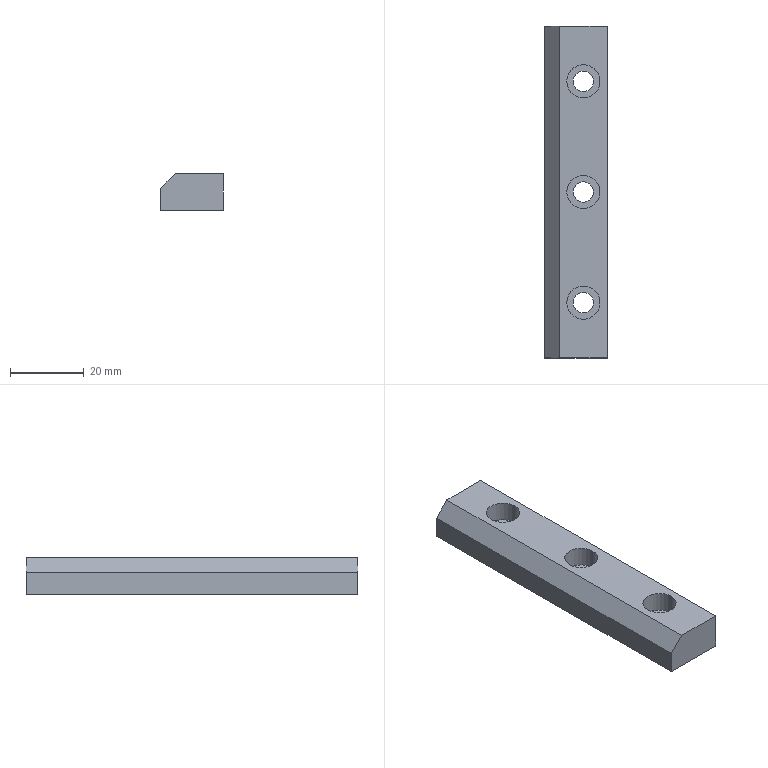Part | STEP file | slide seat cover plate 4 | 1 solid | 22 faces | box 17 x 90 x 10 mm | volume 13210 mm3 | cylinder 12 | plane 10 | commonest cylinder face diameters 5.5 x6 9 x6
STEP:
#1=CARTESIAN_POINT('',(0.,0.,0.));
#2=DIRECTION('',(0.,0.,1.));
#3=DIRECTION('',(1.,0.,0.));
#4=AXIS2_PLACEMENT_3D('',#1,#2,#3);
#5=CARTESIAN_POINT('',(8.148,22.1,4.5));
#6=VERTEX_POINT('',#5);
#7=CARTESIAN_POINT('',(8.148,22.1,10.));
#8=VERTEX_POINT('',#7);
#9=CARTESIAN_POINT('',(8.148,22.1,4.5));
#10=DIRECTION('',(0.,0.,1.));
#11=VECTOR('',#10,1.);
#12=LINE('',#9,#11);
#13=CARTESIAN_POINT('',(3.648,22.1,4.5));
#14=DIRECTION('',(0.,0.,1.));
#15=DIRECTION('',(1.,0.,0.));
#16=AXIS2_PLACEMENT_3D('',#13,#14,#15);
#17=CYLINDRICAL_SURFACE('',#16,4.5);
#18=CARTESIAN_POINT('',(6.283,0.));
#19=DIRECTION('',(0.,1.));
#20=VECTOR('',#19,1.);
#21=LINE('',#18,#20);
#22=(GEOMETRIC_REPRESENTATION_CONTEXT(2)PARAMETRIC_REPRESENTATION_CONTEXT()REPRESENTATION_CONTEXT('',''));
#23=DEFINITIONAL_REPRESENTATION('',(#21),#22);
#24=PCURVE('',#17,#23);
#25=CARTESIAN_POINT('',(3.648,22.1,4.5));
#26=DIRECTION('',(0.,0.,1.));
#27=DIRECTION('',(1.,0.,0.));
#28=AXIS2_PLACEMENT_3D('',#25,#26,#27);
#29=CYLINDRICAL_SURFACE('',#28,4.5);
#30=CARTESIAN_POINT('',(0.,0.));
#31=DIRECTION('',(0.,1.));
#32=VECTOR('',#31,1.);
#33=LINE('',#30,#32);
#34=(GEOMETRIC_REPRESENTATION_CONTEXT(2)PARAMETRIC_REPRESENTATION_CONTEXT()REPRESENTATION_CONTEXT('',''));
#35=DEFINITIONAL_REPRESENTATION('',(#33),#34);
#36=PCURVE('',#29,#35);
#37=SURFACE_CURVE('',#12,(#24,#36),.PCURVE_S1.);
#38=EDGE_CURVE('',#6,#8,#37,.T.);
#39=ORIENTED_EDGE('',*,*,#38,.T.);
#40=CARTESIAN_POINT('',(-0.8518,22.1,10.));
#41=VERTEX_POINT('',#40);
#42=CARTESIAN_POINT('',(3.648,22.1,10.));
#43=DIRECTION('',(0.,0.,1.));
#44=DIRECTION('',(1.,0.,0.));
#45=AXIS2_PLACEMENT_3D('',#42,#43,#44);
#46=CIRCLE('',#45,4.5);
#47=CARTESIAN_POINT('',(0.,5.5));
#48=DIRECTION('',(1.,0.));
#49=VECTOR('',#48,1.);
#50=LINE('',#47,#49);
#51=(GEOMETRIC_REPRESENTATION_CONTEXT(2)PARAMETRIC_REPRESENTATION_CONTEXT()REPRESENTATION_CONTEXT('',''));
#52=DEFINITIONAL_REPRESENTATION('',(#50),#51);
#53=PCURVE('',#17,#52);
#54=CARTESIAN_POINT('',(-6.852,-52.9,10.));
#55=DIRECTION('',(0.,0.,1.));
#56=DIRECTION('',(1.,0.,0.));
#57=AXIS2_PLACEMENT_3D('',#54,#55,#56);
#58=PLANE('',#57);
#59=CARTESIAN_POINT('',(10.5,75.));
#60=DIRECTION('',(1.,0.));
#61=AXIS2_PLACEMENT_2D('',#59,#60);
#62=CIRCLE('',#61,4.5);
#63=(GEOMETRIC_REPRESENTATION_CONTEXT(2)PARAMETRIC_REPRESENTATION_CONTEXT()REPRESENTATION_CONTEXT('',''));
#64=DEFINITIONAL_REPRESENTATION('',(#62),#63);
#65=PCURVE('',#58,#64);
#66=SURFACE_CURVE('',#46,(#53,#65),.PCURVE_S1.);
#67=EDGE_CURVE('',#41,#8,#66,.T.);
#68=ORIENTED_EDGE('',*,*,#67,.F.);
#69=CARTESIAN_POINT('',(-0.8518,22.1,4.5));
#70=VERTEX_POINT('',#69);
#71=CARTESIAN_POINT('',(-0.8518,22.1,4.5));
#72=DIRECTION('',(0.,0.,1.));
#73=VECTOR('',#72,1.);
#74=LINE('',#71,#73);
#75=CARTESIAN_POINT('',(3.142,0.));
#76=DIRECTION('',(0.,1.));
#77=VECTOR('',#76,1.);
#78=LINE('',#75,#77);
#79=(GEOMETRIC_REPRESENTATION_CONTEXT(2)PARAMETRIC_REPRESENTATION_CONTEXT()REPRESENTATION_CONTEXT('',''));
#80=DEFINITIONAL_REPRESENTATION('',(#78),#79);
#81=PCURVE('',#17,#80);
#82=CARTESIAN_POINT('',(3.142,0.));
#83=DIRECTION('',(0.,1.));
#84=VECTOR('',#83,1.);
#85=LINE('',#82,#84);
#86=(GEOMETRIC_REPRESENTATION_CONTEXT(2)PARAMETRIC_REPRESENTATION_CONTEXT()REPRESENTATION_CONTEXT('',''));
#87=DEFINITIONAL_REPRESENTATION('',(#85),#86);
#88=PCURVE('',#29,#87);
#89=SURFACE_CURVE('',#74,(#81,#88),.PCURVE_S1.);
#90=EDGE_CURVE('',#70,#41,#89,.T.);
#91=ORIENTED_EDGE('',*,*,#90,.F.);
#92=CARTESIAN_POINT('',(3.648,22.1,4.5));
#93=DIRECTION('',(0.,0.,1.));
#94=DIRECTION('',(1.,0.,0.));
#95=AXIS2_PLACEMENT_3D('',#92,#93,#94);
#96=CIRCLE('',#95,4.5);
#97=CARTESIAN_POINT('',(0.,0.));
#98=DIRECTION('',(1.,0.));
#99=VECTOR('',#98,1.);
#100=LINE('',#97,#99);
#101=(GEOMETRIC_REPRESENTATION_CONTEXT(2)PARAMETRIC_REPRESENTATION_CONTEXT()REPRESENTATION_CONTEXT('',''));
#102=DEFINITIONAL_REPRESENTATION('',(#100),#101);
#103=PCURVE('',#17,#102);
#104=CARTESIAN_POINT('',(3.648,22.1,4.5));
#105=DIRECTION('',(0.,0.,1.));
#106=DIRECTION('',(1.,0.,0.));
#107=AXIS2_PLACEMENT_3D('',#104,#105,#106);
#108=PLANE('',#107);
#109=CARTESIAN_POINT('',(0.,0.));
#110=DIRECTION('',(1.,0.));
#111=AXIS2_PLACEMENT_2D('',#109,#110);
#112=CIRCLE('',#111,4.5);
#113=(GEOMETRIC_REPRESENTATION_CONTEXT(2)PARAMETRIC_REPRESENTATION_CONTEXT()REPRESENTATION_CONTEXT('',''));
#114=DEFINITIONAL_REPRESENTATION('',(#112),#113);
#115=PCURVE('',#108,#114);
#116=SURFACE_CURVE('',#96,(#103,#115),.PCURVE_S1.);
#117=EDGE_CURVE('',#70,#6,#116,.T.);
#118=ORIENTED_EDGE('',*,*,#117,.T.);
#119=EDGE_LOOP('',(#39,#68,#91,#118));
#120=FACE_BOUND('',#119,.F.);
#121=ADVANCED_FACE('',(#120),#17,.F.);
#122=CARTESIAN_POINT('',(8.148,-7.9,4.5));
#123=VERTEX_POINT('',#122);
#124=CARTESIAN_POINT('',(8.148,-7.9,10.));
#125=VERTEX_POINT('',#124);
#126=CARTESIAN_POINT('',(8.148,-7.9,4.5));
#127=DIRECTION('',(0.,0.,1.));
#128=VECTOR('',#127,1.);
#129=LINE('',#126,#128);
#130=CARTESIAN_POINT('',(3.648,-7.9,4.5));
#131=DIRECTION('',(0.,0.,1.));
#132=DIRECTION('',(1.,0.,0.));
#133=AXIS2_PLACEMENT_3D('',#130,#131,#132);
#134=CYLINDRICAL_SURFACE('',#133,4.5);
#135=CARTESIAN_POINT('',(6.283,0.));
#136=DIRECTION('',(0.,1.));
#137=VECTOR('',#136,1.);
#138=LINE('',#135,#137);
#139=(GEOMETRIC_REPRESENTATION_CONTEXT(2)PARAMETRIC_REPRESENTATION_CONTEXT()REPRESENTATION_CONTEXT('',''));
#140=DEFINITIONAL_REPRESENTATION('',(#138),#139);
#141=PCURVE('',#134,#140);
#142=CARTESIAN_POINT('',(3.648,-7.9,4.5));
#143=DIRECTION('',(0.,0.,1.));
#144=DIRECTION('',(1.,0.,0.));
#145=AXIS2_PLACEMENT_3D('',#142,#143,#144);
#146=CYLINDRICAL_SURFACE('',#145,4.5);
#147=CARTESIAN_POINT('',(0.,0.));
#148=DIRECTION('',(0.,1.));
#149=VECTOR('',#148,1.);
#150=LINE('',#147,#149);
#151=(GEOMETRIC_REPRESENTATION_CONTEXT(2)PARAMETRIC_REPRESENTATION_CONTEXT()REPRESENTATION_CONTEXT('',''));
#152=DEFINITIONAL_REPRESENTATION('',(#150),#151);
#153=PCURVE('',#146,#152);
#154=SURFACE_CURVE('',#129,(#141,#153),.PCURVE_S1.);
#155=EDGE_CURVE('',#123,#125,#154,.T.);
#156=ORIENTED_EDGE('',*,*,#155,.T.);
#157=CARTESIAN_POINT('',(-0.8518,-7.9,10.));
#158=VERTEX_POINT('',#157);
#159=CARTESIAN_POINT('',(3.648,-7.9,10.));
#160=DIRECTION('',(0.,0.,1.));
#161=DIRECTION('',(1.,0.,0.));
#162=AXIS2_PLACEMENT_3D('',#159,#160,#161);
#163=CIRCLE('',#162,4.5);
#164=CARTESIAN_POINT('',(0.,5.5));
#165=DIRECTION('',(1.,0.));
#166=VECTOR('',#165,1.);
#167=LINE('',#164,#166);
#168=(GEOMETRIC_REPRESENTATION_CONTEXT(2)PARAMETRIC_REPRESENTATION_CONTEXT()REPRESENTATION_CONTEXT('',''));
#169=DEFINITIONAL_REPRESENTATION('',(#167),#168);
#170=PCURVE('',#134,#169);
#171=CARTESIAN_POINT('',(10.5,45.));
#172=DIRECTION('',(1.,0.));
#173=AXIS2_PLACEMENT_2D('',#171,#172);
#174=CIRCLE('',#173,4.5);
#175=(GEOMETRIC_REPRESENTATION_CONTEXT(2)PARAMETRIC_REPRESENTATION_CONTEXT()REPRESENTATION_CONTEXT('',''));
#176=DEFINITIONAL_REPRESENTATION('',(#174),#175);
#177=PCURVE('',#58,#176);
#178=SURFACE_CURVE('',#163,(#170,#177),.PCURVE_S1.);
#179=EDGE_CURVE('',#158,#125,#178,.T.);
#180=ORIENTED_EDGE('',*,*,#179,.F.);
#181=CARTESIAN_POINT('',(-0.8518,-7.9,4.5));
#182=VERTEX_POINT('',#181);
#183=CARTESIAN_POINT('',(-0.8518,-7.9,4.5));
#184=DIRECTION('',(0.,0.,1.));
#185=VECTOR('',#184,1.);
#186=LINE('',#183,#185);
#187=CARTESIAN_POINT('',(3.142,0.));
#188=DIRECTION('',(0.,1.));
#189=VECTOR('',#188,1.);
#190=LINE('',#187,#189);
#191=(GEOMETRIC_REPRESENTATION_CONTEXT(2)PARAMETRIC_REPRESENTATION_CONTEXT()REPRESENTATION_CONTEXT('',''));
#192=DEFINITIONAL_REPRESENTATION('',(#190),#191);
#193=PCURVE('',#134,#192);
#194=CARTESIAN_POINT('',(3.142,0.));
#195=DIRECTION('',(0.,1.));
#196=VECTOR('',#195,1.);
#197=LINE('',#194,#196);
#198=(GEOMETRIC_REPRESENTATION_CONTEXT(2)PARAMETRIC_REPRESENTATION_CONTEXT()REPRESENTATION_CONTEXT('',''));
#199=DEFINITIONAL_REPRESENTATION('',(#197),#198);
#200=PCURVE('',#146,#199);
#201=SURFACE_CURVE('',#186,(#193,#200),.PCURVE_S1.);
#202=EDGE_CURVE('',#182,#158,#201,.T.);
#203=ORIENTED_EDGE('',*,*,#202,.F.);
#204=CARTESIAN_POINT('',(3.648,-7.9,4.5));
#205=DIRECTION('',(0.,0.,1.));
#206=DIRECTION('',(1.,0.,0.));
#207=AXIS2_PLACEMENT_3D('',#204,#205,#206);
#208=CIRCLE('',#207,4.5);
#209=CARTESIAN_POINT('',(0.,0.));
#210=DIRECTION('',(1.,0.));
#211=VECTOR('',#210,1.);
#212=LINE('',#209,#211);
#213=(GEOMETRIC_REPRESENTATION_CONTEXT(2)PARAMETRIC_REPRESENTATION_CONTEXT()REPRESENTATION_CONTEXT('',''));
#214=DEFINITIONAL_REPRESENTATION('',(#212),#213);
#215=PCURVE('',#134,#214);
#216=CARTESIAN_POINT('',(3.648,-7.9,4.5));
#217=DIRECTION('',(0.,0.,1.));
#218=DIRECTION('',(1.,0.,0.));
#219=AXIS2_PLACEMENT_3D('',#216,#217,#218);
#220=PLANE('',#219);
#221=CARTESIAN_POINT('',(0.,0.));
#222=DIRECTION('',(1.,0.));
#223=AXIS2_PLACEMENT_2D('',#221,#222);
#224=CIRCLE('',#223,4.5);
#225=(GEOMETRIC_REPRESENTATION_CONTEXT(2)PARAMETRIC_REPRESENTATION_CONTEXT()REPRESENTATION_CONTEXT('',''));
#226=DEFINITIONAL_REPRESENTATION('',(#224),#225);
#227=PCURVE('',#220,#226);
#228=SURFACE_CURVE('',#208,(#215,#227),.PCURVE_S1.);
#229=EDGE_CURVE('',#182,#123,#228,.T.);
#230=ORIENTED_EDGE('',*,*,#229,.T.);
#231=EDGE_LOOP('',(#156,#180,#203,#230));
#232=FACE_BOUND('',#231,.F.);
#233=ADVANCED_FACE('',(#232),#134,.F.);
#234=CARTESIAN_POINT('',(8.148,-37.9,4.5));
#235=VERTEX_POINT('',#234);
#236=CARTESIAN_POINT('',(8.148,-37.9,10.));
#237=VERTEX_POINT('',#236);
#238=CARTESIAN_POINT('',(8.148,-37.9,4.5));
#239=DIRECTION('',(0.,0.,1.));
#240=VECTOR('',#239,1.);
#241=LINE('',#238,#240);
#242=CARTESIAN_POINT('',(3.648,-37.9,4.5));
#243=DIRECTION('',(0.,0.,1.));
#244=DIRECTION('',(1.,0.,0.));
#245=AXIS2_PLACEMENT_3D('',#242,#243,#244);
#246=CYLINDRICAL_SURFACE('',#245,4.5);
#247=CARTESIAN_POINT('',(6.283,0.));
#248=DIRECTION('',(0.,1.));
#249=VECTOR('',#248,1.);
#250=LINE('',#247,#249);
#251=(GEOMETRIC_REPRESENTATION_CONTEXT(2)PARAMETRIC_REPRESENTATION_CONTEXT()REPRESENTATION_CONTEXT('',''));
#252=DEFINITIONAL_REPRESENTATION('',(#250),#251);
#253=PCURVE('',#246,#252);
#254=CARTESIAN_POINT('',(3.648,-37.9,4.5));
#255=DIRECTION('',(0.,0.,1.));
#256=DIRECTION('',(1.,0.,0.));
#257=AXIS2_PLACEMENT_3D('',#254,#255,#256);
#258=CYLINDRICAL_SURFACE('',#257,4.5);
#259=CARTESIAN_POINT('',(0.,0.));
#260=DIRECTION('',(0.,1.));
#261=VECTOR('',#260,1.);
#262=LINE('',#259,#261);
#263=(GEOMETRIC_REPRESENTATION_CONTEXT(2)PARAMETRIC_REPRESENTATION_CONTEXT()REPRESENTATION_CONTEXT('',''));
#264=DEFINITIONAL_REPRESENTATION('',(#262),#263);
#265=PCURVE('',#258,#264);
#266=SURFACE_CURVE('',#241,(#253,#265),.PCURVE_S1.);
#267=EDGE_CURVE('',#235,#237,#266,.T.);
#268=ORIENTED_EDGE('',*,*,#267,.T.);
#269=CARTESIAN_POINT('',(-0.8518,-37.9,10.));
#270=VERTEX_POINT('',#269);
#271=CARTESIAN_POINT('',(3.648,-37.9,10.));
#272=DIRECTION('',(0.,0.,1.));
#273=DIRECTION('',(1.,0.,0.));
#274=AXIS2_PLACEMENT_3D('',#271,#272,#273);
#275=CIRCLE('',#274,4.5);
#276=CARTESIAN_POINT('',(0.,5.5));
#277=DIRECTION('',(1.,0.));
#278=VECTOR('',#277,1.);
#279=LINE('',#276,#278);
#280=(GEOMETRIC_REPRESENTATION_CONTEXT(2)PARAMETRIC_REPRESENTATION_CONTEXT()REPRESENTATION_CONTEXT('',''));
#281=DEFINITIONAL_REPRESENTATION('',(#279),#280);
#282=PCURVE('',#246,#281);
#283=CARTESIAN_POINT('',(10.5,15.));
#284=DIRECTION('',(1.,0.));
#285=AXIS2_PLACEMENT_2D('',#283,#284);
#286=CIRCLE('',#285,4.5);
#287=(GEOMETRIC_REPRESENTATION_CONTEXT(2)PARAMETRIC_REPRESENTATION_CONTEXT()REPRESENTATION_CONTEXT('',''));
#288=DEFINITIONAL_REPRESENTATION('',(#286),#287);
#289=PCURVE('',#58,#288);
#290=SURFACE_CURVE('',#275,(#282,#289),.PCURVE_S1.);
#291=EDGE_CURVE('',#270,#237,#290,.T.);
#292=ORIENTED_EDGE('',*,*,#291,.F.);
#293=CARTESIAN_POINT('',(-0.8518,-37.9,4.5));
#294=VERTEX_POINT('',#293);
#295=CARTESIAN_POINT('',(-0.8518,-37.9,4.5));
#296=DIRECTION('',(0.,0.,1.));
#297=VECTOR('',#296,1.);
#298=LINE('',#295,#297);
#299=CARTESIAN_POINT('',(3.142,0.));
#300=DIRECTION('',(0.,1.));
#301=VECTOR('',#300,1.);
#302=LINE('',#299,#301);
#303=(GEOMETRIC_REPRESENTATION_CONTEXT(2)PARAMETRIC_REPRESENTATION_CONTEXT()REPRESENTATION_CONTEXT('',''));
#304=DEFINITIONAL_REPRESENTATION('',(#302),#303);
#305=PCURVE('',#246,#304);
#306=CARTESIAN_POINT('',(3.142,0.));
#307=DIRECTION('',(0.,1.));
#308=VECTOR('',#307,1.);
#309=LINE('',#306,#308);
#310=(GEOMETRIC_REPRESENTATION_CONTEXT(2)PARAMETRIC_REPRESENTATION_CONTEXT()REPRESENTATION_CONTEXT('',''));
#311=DEFINITIONAL_REPRESENTATION('',(#309),#310);
#312=PCURVE('',#258,#311);
#313=SURFACE_CURVE('',#298,(#305,#312),.PCURVE_S1.);
#314=EDGE_CURVE('',#294,#270,#313,.T.);
#315=ORIENTED_EDGE('',*,*,#314,.F.);
#316=CARTESIAN_POINT('',(3.648,-37.9,4.5));
#317=DIRECTION('',(0.,0.,1.));
#318=DIRECTION('',(1.,0.,0.));
#319=AXIS2_PLACEMENT_3D('',#316,#317,#318);
#320=CIRCLE('',#319,4.5);
#321=CARTESIAN_POINT('',(0.,0.));
#322=DIRECTION('',(1.,0.));
#323=VECTOR('',#322,1.);
#324=LINE('',#321,#323);
#325=(GEOMETRIC_REPRESENTATION_CONTEXT(2)PARAMETRIC_REPRESENTATION_CONTEXT()REPRESENTATION_CONTEXT('',''));
#326=DEFINITIONAL_REPRESENTATION('',(#324),#325);
#327=PCURVE('',#246,#326);
#328=CARTESIAN_POINT('',(3.648,-37.9,4.5));
#329=DIRECTION('',(0.,0.,1.));
#330=DIRECTION('',(1.,0.,0.));
#331=AXIS2_PLACEMENT_3D('',#328,#329,#330);
#332=PLANE('',#331);
#333=CARTESIAN_POINT('',(0.,0.));
#334=DIRECTION('',(1.,0.));
#335=AXIS2_PLACEMENT_2D('',#333,#334);
#336=CIRCLE('',#335,4.5);
#337=(GEOMETRIC_REPRESENTATION_CONTEXT(2)PARAMETRIC_REPRESENTATION_CONTEXT()REPRESENTATION_CONTEXT('',''));
#338=DEFINITIONAL_REPRESENTATION('',(#336),#337);
#339=PCURVE('',#332,#338);
#340=SURFACE_CURVE('',#320,(#327,#339),.PCURVE_S1.);
#341=EDGE_CURVE('',#294,#235,#340,.T.);
#342=ORIENTED_EDGE('',*,*,#341,.T.);
#343=EDGE_LOOP('',(#268,#292,#315,#342));
#344=FACE_BOUND('',#343,.F.);
#345=ADVANCED_FACE('',(#344),#246,.F.);
#346=CARTESIAN_POINT('',(0.8982,-37.9,4.5));
#347=VERTEX_POINT('',#346);
#348=CARTESIAN_POINT('',(0.8982,-37.9,0.));
#349=VERTEX_POINT('',#348);
#350=CARTESIAN_POINT('',(0.8982,-37.9,10.));
#351=DIRECTION('',(0.,0.,-1.));
#352=VECTOR('',#351,1.);
#353=LINE('',#350,#352);
#354=CARTESIAN_POINT('',(3.648,-37.9,10.));
#355=DIRECTION('',(0.,0.,-1.));
#356=DIRECTION('',(-1.,0.,0.));
#357=AXIS2_PLACEMENT_3D('',#354,#355,#356);
#358=CYLINDRICAL_SURFACE('',#357,2.75);
#359=CARTESIAN_POINT('',(6.283,0.));
#360=DIRECTION('',(0.,1.));
#361=VECTOR('',#360,1.);
#362=LINE('',#359,#361);
#363=(GEOMETRIC_REPRESENTATION_CONTEXT(2)PARAMETRIC_REPRESENTATION_CONTEXT()REPRESENTATION_CONTEXT('',''));
#364=DEFINITIONAL_REPRESENTATION('',(#362),#363);
#365=PCURVE('',#358,#364);
#366=CARTESIAN_POINT('',(3.648,-37.9,10.));
#367=DIRECTION('',(0.,0.,-1.));
#368=DIRECTION('',(-1.,0.,0.));
#369=AXIS2_PLACEMENT_3D('',#366,#367,#368);
#370=CYLINDRICAL_SURFACE('',#369,2.75);
#371=CARTESIAN_POINT('',(0.,0.));
#372=DIRECTION('',(0.,1.));
#373=VECTOR('',#372,1.);
#374=LINE('',#371,#373);
#375=(GEOMETRIC_REPRESENTATION_CONTEXT(2)PARAMETRIC_REPRESENTATION_CONTEXT()REPRESENTATION_CONTEXT('',''));
#376=DEFINITIONAL_REPRESENTATION('',(#374),#375);
#377=PCURVE('',#370,#376);
#378=SURFACE_CURVE('',#353,(#365,#377),.PCURVE_S1.);
#379=EDGE_CURVE('',#347,#349,#378,.T.);
#380=ORIENTED_EDGE('',*,*,#379,.T.);
#381=CARTESIAN_POINT('',(6.398,-37.9,0.));
#382=VERTEX_POINT('',#381);
#383=CARTESIAN_POINT('',(3.648,-37.9,0.));
#384=DIRECTION('',(0.,0.,1.));
#385=DIRECTION('',(1.,0.,0.));
#386=AXIS2_PLACEMENT_3D('',#383,#384,#385);
#387=CIRCLE('',#386,2.75);
#388=CARTESIAN_POINT('',(9.425,10.));
#389=DIRECTION('',(-1.,0.));
#390=VECTOR('',#389,1.);
#391=LINE('',#388,#390);
#392=(GEOMETRIC_REPRESENTATION_CONTEXT(2)PARAMETRIC_REPRESENTATION_CONTEXT()REPRESENTATION_CONTEXT('',''));
#393=DEFINITIONAL_REPRESENTATION('',(#391),#392);
#394=PCURVE('',#358,#393);
#395=CARTESIAN_POINT('',(-6.852,-52.9,0.));
#396=DIRECTION('',(0.,0.,1.));
#397=DIRECTION('',(1.,0.,0.));
#398=AXIS2_PLACEMENT_3D('',#395,#396,#397);
#399=PLANE('',#398);
#400=CARTESIAN_POINT('',(10.5,15.));
#401=DIRECTION('',(1.,0.));
#402=AXIS2_PLACEMENT_2D('',#400,#401);
#403=CIRCLE('',#402,2.75);
#404=(GEOMETRIC_REPRESENTATION_CONTEXT(2)PARAMETRIC_REPRESENTATION_CONTEXT()REPRESENTATION_CONTEXT('',''));
#405=DEFINITIONAL_REPRESENTATION('',(#403),#404);
#406=PCURVE('',#399,#405);
#407=SURFACE_CURVE('',#387,(#394,#406),.PCURVE_S1.);
#408=EDGE_CURVE('',#349,#382,#407,.T.);
#409=ORIENTED_EDGE('',*,*,#408,.T.);
#410=CARTESIAN_POINT('',(6.398,-37.9,4.5));
#411=VERTEX_POINT('',#410);
#412=CARTESIAN_POINT('',(6.398,-37.9,10.));
#413=DIRECTION('',(0.,0.,-1.));
#414=VECTOR('',#413,1.);
#415=LINE('',#412,#414);
#416=CARTESIAN_POINT('',(3.142,0.));
#417=DIRECTION('',(0.,1.));
#418=VECTOR('',#417,1.);
#419=LINE('',#416,#418);
#420=(GEOMETRIC_REPRESENTATION_CONTEXT(2)PARAMETRIC_REPRESENTATION_CONTEXT()REPRESENTATION_CONTEXT('',''));
#421=DEFINITIONAL_REPRESENTATION('',(#419),#420);
#422=PCURVE('',#358,#421);
#423=CARTESIAN_POINT('',(3.142,0.));
#424=DIRECTION('',(0.,1.));
#425=VECTOR('',#424,1.);
#426=LINE('',#423,#425);
#427=(GEOMETRIC_REPRESENTATION_CONTEXT(2)PARAMETRIC_REPRESENTATION_CONTEXT()REPRESENTATION_CONTEXT('',''));
#428=DEFINITIONAL_REPRESENTATION('',(#426),#427);
#429=PCURVE('',#370,#428);
#430=SURFACE_CURVE('',#415,(#422,#429),.PCURVE_S1.);
#431=EDGE_CURVE('',#411,#382,#430,.T.);
#432=ORIENTED_EDGE('',*,*,#431,.F.);
#433=CARTESIAN_POINT('',(3.648,-37.9,4.5));
#434=DIRECTION('',(0.,0.,1.));
#435=DIRECTION('',(1.,0.,0.));
#436=AXIS2_PLACEMENT_3D('',#433,#434,#435);
#437=CIRCLE('',#436,2.75);
#438=CARTESIAN_POINT('',(9.425,5.5));
#439=DIRECTION('',(-1.,0.));
#440=VECTOR('',#439,1.);
#441=LINE('',#438,#440);
#442=(GEOMETRIC_REPRESENTATION_CONTEXT(2)PARAMETRIC_REPRESENTATION_CONTEXT()REPRESENTATION_CONTEXT('',''));
#443=DEFINITIONAL_REPRESENTATION('',(#441),#442);
#444=PCURVE('',#358,#443);
#445=CARTESIAN_POINT('',(0.,0.));
#446=DIRECTION('',(1.,0.));
#447=AXIS2_PLACEMENT_2D('',#445,#446);
#448=CIRCLE('',#447,2.75);
#449=(GEOMETRIC_REPRESENTATION_CONTEXT(2)PARAMETRIC_REPRESENTATION_CONTEXT()REPRESENTATION_CONTEXT('',''));
#450=DEFINITIONAL_REPRESENTATION('',(#448),#449);
#451=PCURVE('',#332,#450);
#452=SURFACE_CURVE('',#437,(#444,#451),.PCURVE_S1.);
#453=EDGE_CURVE('',#347,#411,#452,.T.);
#454=ORIENTED_EDGE('',*,*,#453,.F.);
#455=EDGE_LOOP('',(#380,#409,#432,#454));
#456=FACE_BOUND('',#455,.F.);
#457=ADVANCED_FACE('',(#456),#358,.F.);
#458=CARTESIAN_POINT('',(0.8982,-7.9,4.5));
#459=VERTEX_POINT('',#458);
#460=CARTESIAN_POINT('',(0.8982,-7.9,0.));
#461=VERTEX_POINT('',#460);
#462=CARTESIAN_POINT('',(0.8982,-7.9,10.));
#463=DIRECTION('',(0.,0.,-1.));
#464=VECTOR('',#463,1.);
#465=LINE('',#462,#464);
#466=CARTESIAN_POINT('',(3.648,-7.9,10.));
#467=DIRECTION('',(0.,0.,-1.));
#468=DIRECTION('',(-1.,0.,0.));
#469=AXIS2_PLACEMENT_3D('',#466,#467,#468);
#470=CYLINDRICAL_SURFACE('',#469,2.75);
#471=CARTESIAN_POINT('',(6.283,0.));
#472=DIRECTION('',(0.,1.));
#473=VECTOR('',#472,1.);
#474=LINE('',#471,#473);
#475=(GEOMETRIC_REPRESENTATION_CONTEXT(2)PARAMETRIC_REPRESENTATION_CONTEXT()REPRESENTATION_CONTEXT('',''));
#476=DEFINITIONAL_REPRESENTATION('',(#474),#475);
#477=PCURVE('',#470,#476);
#478=CARTESIAN_POINT('',(3.648,-7.9,10.));
#479=DIRECTION('',(0.,0.,-1.));
#480=DIRECTION('',(-1.,0.,0.));
#481=AXIS2_PLACEMENT_3D('',#478,#479,#480);
#482=CYLINDRICAL_SURFACE('',#481,2.75);
#483=CARTESIAN_POINT('',(0.,0.));
#484=DIRECTION('',(0.,1.));
#485=VECTOR('',#484,1.);
#486=LINE('',#483,#485);
#487=(GEOMETRIC_REPRESENTATION_CONTEXT(2)PARAMETRIC_REPRESENTATION_CONTEXT()REPRESENTATION_CONTEXT('',''));
#488=DEFINITIONAL_REPRESENTATION('',(#486),#487);
#489=PCURVE('',#482,#488);
#490=SURFACE_CURVE('',#465,(#477,#489),.PCURVE_S1.);
#491=EDGE_CURVE('',#459,#461,#490,.T.);
#492=ORIENTED_EDGE('',*,*,#491,.T.);
#493=CARTESIAN_POINT('',(6.398,-7.9,0.));
#494=VERTEX_POINT('',#493);
#495=CARTESIAN_POINT('',(3.648,-7.9,0.));
#496=DIRECTION('',(0.,0.,1.));
#497=DIRECTION('',(1.,0.,0.));
#498=AXIS2_PLACEMENT_3D('',#495,#496,#497);
#499=CIRCLE('',#498,2.75);
#500=CARTESIAN_POINT('',(9.425,10.));
#501=DIRECTION('',(-1.,0.));
#502=VECTOR('',#501,1.);
#503=LINE('',#500,#502);
#504=(GEOMETRIC_REPRESENTATION_CONTEXT(2)PARAMETRIC_REPRESENTATION_CONTEXT()REPRESENTATION_CONTEXT('',''));
#505=DEFINITIONAL_REPRESENTATION('',(#503),#504);
#506=PCURVE('',#470,#505);
#507=CARTESIAN_POINT('',(10.5,45.));
#508=DIRECTION('',(1.,0.));
#509=AXIS2_PLACEMENT_2D('',#507,#508);
#510=CIRCLE('',#509,2.75);
#511=(GEOMETRIC_REPRESENTATION_CONTEXT(2)PARAMETRIC_REPRESENTATION_CONTEXT()REPRESENTATION_CONTEXT('',''));
#512=DEFINITIONAL_REPRESENTATION('',(#510),#511);
#513=PCURVE('',#399,#512);
#514=SURFACE_CURVE('',#499,(#506,#513),.PCURVE_S1.);
#515=EDGE_CURVE('',#461,#494,#514,.T.);
#516=ORIENTED_EDGE('',*,*,#515,.T.);
#517=CARTESIAN_POINT('',(6.398,-7.9,4.5));
#518=VERTEX_POINT('',#517);
#519=CARTESIAN_POINT('',(6.398,-7.9,10.));
#520=DIRECTION('',(0.,0.,-1.));
#521=VECTOR('',#520,1.);
#522=LINE('',#519,#521);
#523=CARTESIAN_POINT('',(3.142,0.));
#524=DIRECTION('',(0.,1.));
#525=VECTOR('',#524,1.);
#526=LINE('',#523,#525);
#527=(GEOMETRIC_REPRESENTATION_CONTEXT(2)PARAMETRIC_REPRESENTATION_CONTEXT()REPRESENTATION_CONTEXT('',''));
#528=DEFINITIONAL_REPRESENTATION('',(#526),#527);
#529=PCURVE('',#470,#528);
#530=CARTESIAN_POINT('',(3.142,0.));
#531=DIRECTION('',(0.,1.));
#532=VECTOR('',#531,1.);
#533=LINE('',#530,#532);
#534=(GEOMETRIC_REPRESENTATION_CONTEXT(2)PARAMETRIC_REPRESENTATION_CONTEXT()REPRESENTATION_CONTEXT('',''));
#535=DEFINITIONAL_REPRESENTATION('',(#533),#534);
#536=PCURVE('',#482,#535);
#537=SURFACE_CURVE('',#522,(#529,#536),.PCURVE_S1.);
#538=EDGE_CURVE('',#518,#494,#537,.T.);
#539=ORIENTED_EDGE('',*,*,#538,.F.);
#540=CARTESIAN_POINT('',(3.648,-7.9,4.5));
#541=DIRECTION('',(0.,0.,1.));
#542=DIRECTION('',(1.,0.,0.));
#543=AXIS2_PLACEMENT_3D('',#540,#541,#542);
#544=CIRCLE('',#543,2.75);
#545=CARTESIAN_POINT('',(9.425,5.5));
#546=DIRECTION('',(-1.,0.));
#547=VECTOR('',#546,1.);
#548=LINE('',#545,#547);
#549=(GEOMETRIC_REPRESENTATION_CONTEXT(2)PARAMETRIC_REPRESENTATION_CONTEXT()REPRESENTATION_CONTEXT('',''));
#550=DEFINITIONAL_REPRESENTATION('',(#548),#549);
#551=PCURVE('',#470,#550);
#552=CARTESIAN_POINT('',(0.,0.));
#553=DIRECTION('',(1.,0.));
#554=AXIS2_PLACEMENT_2D('',#552,#553);
#555=CIRCLE('',#554,2.75);
#556=(GEOMETRIC_REPRESENTATION_CONTEXT(2)PARAMETRIC_REPRESENTATION_CONTEXT()REPRESENTATION_CONTEXT('',''));
#557=DEFINITIONAL_REPRESENTATION('',(#555),#556);
#558=PCURVE('',#220,#557);
#559=SURFACE_CURVE('',#544,(#551,#558),.PCURVE_S1.);
#560=EDGE_CURVE('',#459,#518,#559,.T.);
#561=ORIENTED_EDGE('',*,*,#560,.F.);
#562=EDGE_LOOP('',(#492,#516,#539,#561));
#563=FACE_BOUND('',#562,.F.);
#564=ADVANCED_FACE('',(#563),#470,.F.);
#565=CARTESIAN_POINT('',(0.8982,22.1,4.5));
#566=VERTEX_POINT('',#565);
#567=CARTESIAN_POINT('',(0.8982,22.1,0.));
#568=VERTEX_POINT('',#567);
#569=CARTESIAN_POINT('',(0.8982,22.1,10.));
#570=DIRECTION('',(0.,0.,-1.));
#571=VECTOR('',#570,1.);
#572=LINE('',#569,#571);
#573=CARTESIAN_POINT('',(3.648,22.1,10.));
#574=DIRECTION('',(0.,0.,-1.));
#575=DIRECTION('',(-1.,0.,0.));
#576=AXIS2_PLACEMENT_3D('',#573,#574,#575);
#577=CYLINDRICAL_SURFACE('',#576,2.75);
#578=CARTESIAN_POINT('',(6.283,0.));
#579=DIRECTION('',(0.,1.));
#580=VECTOR('',#579,1.);
#581=LINE('',#578,#580);
#582=(GEOMETRIC_REPRESENTATION_CONTEXT(2)PARAMETRIC_REPRESENTATION_CONTEXT()REPRESENTATION_CONTEXT('',''));
#583=DEFINITIONAL_REPRESENTATION('',(#581),#582);
#584=PCURVE('',#577,#583);
#585=CARTESIAN_POINT('',(3.648,22.1,10.));
#586=DIRECTION('',(0.,0.,-1.));
#587=DIRECTION('',(-1.,0.,0.));
#588=AXIS2_PLACEMENT_3D('',#585,#586,#587);
#589=CYLINDRICAL_SURFACE('',#588,2.75);
#590=CARTESIAN_POINT('',(0.,0.));
#591=DIRECTION('',(0.,1.));
#592=VECTOR('',#591,1.);
#593=LINE('',#590,#592);
#594=(GEOMETRIC_REPRESENTATION_CONTEXT(2)PARAMETRIC_REPRESENTATION_CONTEXT()REPRESENTATION_CONTEXT('',''));
#595=DEFINITIONAL_REPRESENTATION('',(#593),#594);
#596=PCURVE('',#589,#595);
#597=SURFACE_CURVE('',#572,(#584,#596),.PCURVE_S1.);
#598=EDGE_CURVE('',#566,#568,#597,.T.);
#599=ORIENTED_EDGE('',*,*,#598,.T.);
#600=CARTESIAN_POINT('',(6.398,22.1,0.));
#601=VERTEX_POINT('',#600);
#602=CARTESIAN_POINT('',(3.648,22.1,0.));
#603=DIRECTION('',(0.,0.,1.));
#604=DIRECTION('',(1.,0.,0.));
#605=AXIS2_PLACEMENT_3D('',#602,#603,#604);
#606=CIRCLE('',#605,2.75);
#607=CARTESIAN_POINT('',(9.425,10.));
#608=DIRECTION('',(-1.,0.));
#609=VECTOR('',#608,1.);
#610=LINE('',#607,#609);
#611=(GEOMETRIC_REPRESENTATION_CONTEXT(2)PARAMETRIC_REPRESENTATION_CONTEXT()REPRESENTATION_CONTEXT('',''));
#612=DEFINITIONAL_REPRESENTATION('',(#610),#611);
#613=PCURVE('',#577,#612);
#614=CARTESIAN_POINT('',(10.5,75.));
#615=DIRECTION('',(1.,0.));
#616=AXIS2_PLACEMENT_2D('',#614,#615);
#617=CIRCLE('',#616,2.75);
#618=(GEOMETRIC_REPRESENTATION_CONTEXT(2)PARAMETRIC_REPRESENTATION_CONTEXT()REPRESENTATION_CONTEXT('',''));
#619=DEFINITIONAL_REPRESENTATION('',(#617),#618);
#620=PCURVE('',#399,#619);
#621=SURFACE_CURVE('',#606,(#613,#620),.PCURVE_S1.);
#622=EDGE_CURVE('',#568,#601,#621,.T.);
#623=ORIENTED_EDGE('',*,*,#622,.T.);
#624=CARTESIAN_POINT('',(6.398,22.1,4.5));
#625=VERTEX_POINT('',#624);
#626=CARTESIAN_POINT('',(6.398,22.1,10.));
#627=DIRECTION('',(0.,0.,-1.));
#628=VECTOR('',#627,1.);
#629=LINE('',#626,#628);
#630=CARTESIAN_POINT('',(3.142,0.));
#631=DIRECTION('',(0.,1.));
#632=VECTOR('',#631,1.);
#633=LINE('',#630,#632);
#634=(GEOMETRIC_REPRESENTATION_CONTEXT(2)PARAMETRIC_REPRESENTATION_CONTEXT()REPRESENTATION_CONTEXT('',''));
#635=DEFINITIONAL_REPRESENTATION('',(#633),#634);
#636=PCURVE('',#577,#635);
#637=CARTESIAN_POINT('',(3.142,0.));
#638=DIRECTION('',(0.,1.));
#639=VECTOR('',#638,1.);
#640=LINE('',#637,#639);
#641=(GEOMETRIC_REPRESENTATION_CONTEXT(2)PARAMETRIC_REPRESENTATION_CONTEXT()REPRESENTATION_CONTEXT('',''));
#642=DEFINITIONAL_REPRESENTATION('',(#640),#641);
#643=PCURVE('',#589,#642);
#644=SURFACE_CURVE('',#629,(#636,#643),.PCURVE_S1.);
#645=EDGE_CURVE('',#625,#601,#644,.T.);
#646=ORIENTED_EDGE('',*,*,#645,.F.);
#647=CARTESIAN_POINT('',(3.648,22.1,4.5));
#648=DIRECTION('',(0.,0.,1.));
#649=DIRECTION('',(1.,0.,0.));
#650=AXIS2_PLACEMENT_3D('',#647,#648,#649);
#651=CIRCLE('',#650,2.75);
#652=CARTESIAN_POINT('',(9.425,5.5));
#653=DIRECTION('',(-1.,0.));
#654=VECTOR('',#653,1.);
#655=LINE('',#652,#654);
#656=(GEOMETRIC_REPRESENTATION_CONTEXT(2)PARAMETRIC_REPRESENTATION_CONTEXT()REPRESENTATION_CONTEXT('',''));
#657=DEFINITIONAL_REPRESENTATION('',(#655),#656);
#658=PCURVE('',#577,#657);
#659=CARTESIAN_POINT('',(0.,0.));
#660=DIRECTION('',(1.,0.));
#661=AXIS2_PLACEMENT_2D('',#659,#660);
#662=CIRCLE('',#661,2.75);
#663=(GEOMETRIC_REPRESENTATION_CONTEXT(2)PARAMETRIC_REPRESENTATION_CONTEXT()REPRESENTATION_CONTEXT('',''));
#664=DEFINITIONAL_REPRESENTATION('',(#662),#663);
#665=PCURVE('',#108,#664);
#666=SURFACE_CURVE('',#651,(#658,#665),.PCURVE_S1.);
#667=EDGE_CURVE('',#566,#625,#666,.T.);
#668=ORIENTED_EDGE('',*,*,#667,.F.);
#669=EDGE_LOOP('',(#599,#623,#646,#668));
#670=FACE_BOUND('',#669,.F.);
#671=ADVANCED_FACE('',(#670),#577,.F.);
#672=CARTESIAN_POINT('',(3.648,22.1,0.));
#673=DIRECTION('',(0.,0.,1.));
#674=DIRECTION('',(1.,0.,0.));
#675=AXIS2_PLACEMENT_3D('',#672,#673,#674);
#676=CIRCLE('',#675,2.75);
#677=CARTESIAN_POINT('',(3.142,10.));
#678=DIRECTION('',(-1.,0.));
#679=VECTOR('',#678,1.);
#680=LINE('',#677,#679);
#681=(GEOMETRIC_REPRESENTATION_CONTEXT(2)PARAMETRIC_REPRESENTATION_CONTEXT()REPRESENTATION_CONTEXT('',''));
#682=DEFINITIONAL_REPRESENTATION('',(#680),#681);
#683=PCURVE('',#589,#682);
#684=CARTESIAN_POINT('',(10.5,75.));
#685=DIRECTION('',(1.,0.));
#686=AXIS2_PLACEMENT_2D('',#684,#685);
#687=CIRCLE('',#686,2.75);
#688=(GEOMETRIC_REPRESENTATION_CONTEXT(2)PARAMETRIC_REPRESENTATION_CONTEXT()REPRESENTATION_CONTEXT('',''));
#689=DEFINITIONAL_REPRESENTATION('',(#687),#688);
#690=PCURVE('',#399,#689);
#691=SURFACE_CURVE('',#676,(#683,#690),.PCURVE_S1.);
#692=EDGE_CURVE('',#601,#568,#691,.T.);
#693=ORIENTED_EDGE('',*,*,#692,.T.);
#694=ORIENTED_EDGE('',*,*,#598,.F.);
#695=CARTESIAN_POINT('',(3.648,22.1,4.5));
#696=DIRECTION('',(0.,0.,1.));
#697=DIRECTION('',(1.,0.,0.));
#698=AXIS2_PLACEMENT_3D('',#695,#696,#697);
#699=CIRCLE('',#698,2.75);
#700=CARTESIAN_POINT('',(3.142,5.5));
#701=DIRECTION('',(-1.,0.));
#702=VECTOR('',#701,1.);
#703=LINE('',#700,#702);
#704=(GEOMETRIC_REPRESENTATION_CONTEXT(2)PARAMETRIC_REPRESENTATION_CONTEXT()REPRESENTATION_CONTEXT('',''));
#705=DEFINITIONAL_REPRESENTATION('',(#703),#704);
#706=PCURVE('',#589,#705);
#707=CARTESIAN_POINT('',(0.,0.));
#708=DIRECTION('',(1.,0.));
#709=AXIS2_PLACEMENT_2D('',#707,#708);
#710=CIRCLE('',#709,2.75);
#711=(GEOMETRIC_REPRESENTATION_CONTEXT(2)PARAMETRIC_REPRESENTATION_CONTEXT()REPRESENTATION_CONTEXT('',''));
#712=DEFINITIONAL_REPRESENTATION('',(#710),#711);
#713=PCURVE('',#108,#712);
#714=SURFACE_CURVE('',#699,(#706,#713),.PCURVE_S1.);
#715=EDGE_CURVE('',#625,#566,#714,.T.);
#716=ORIENTED_EDGE('',*,*,#715,.F.);
#717=ORIENTED_EDGE('',*,*,#645,.T.);
#718=EDGE_LOOP('',(#693,#694,#716,#717));
#719=FACE_BOUND('',#718,.F.);
#720=ADVANCED_FACE('',(#719),#589,.F.);
#721=CARTESIAN_POINT('',(3.648,-7.9,0.));
#722=DIRECTION('',(0.,0.,1.));
#723=DIRECTION('',(1.,0.,0.));
#724=AXIS2_PLACEMENT_3D('',#721,#722,#723);
#725=CIRCLE('',#724,2.75);
#726=CARTESIAN_POINT('',(3.142,10.));
#727=DIRECTION('',(-1.,0.));
#728=VECTOR('',#727,1.);
#729=LINE('',#726,#728);
#730=(GEOMETRIC_REPRESENTATION_CONTEXT(2)PARAMETRIC_REPRESENTATION_CONTEXT()REPRESENTATION_CONTEXT('',''));
#731=DEFINITIONAL_REPRESENTATION('',(#729),#730);
#732=PCURVE('',#482,#731);
#733=CARTESIAN_POINT('',(10.5,45.));
#734=DIRECTION('',(1.,0.));
#735=AXIS2_PLACEMENT_2D('',#733,#734);
#736=CIRCLE('',#735,2.75);
#737=(GEOMETRIC_REPRESENTATION_CONTEXT(2)PARAMETRIC_REPRESENTATION_CONTEXT()REPRESENTATION_CONTEXT('',''));
#738=DEFINITIONAL_REPRESENTATION('',(#736),#737);
#739=PCURVE('',#399,#738);
#740=SURFACE_CURVE('',#725,(#732,#739),.PCURVE_S1.);
#741=EDGE_CURVE('',#494,#461,#740,.T.);
#742=ORIENTED_EDGE('',*,*,#741,.T.);
#743=ORIENTED_EDGE('',*,*,#491,.F.);
#744=CARTESIAN_POINT('',(3.648,-7.9,4.5));
#745=DIRECTION('',(0.,0.,1.));
#746=DIRECTION('',(1.,0.,0.));
#747=AXIS2_PLACEMENT_3D('',#744,#745,#746);
#748=CIRCLE('',#747,2.75);
#749=CARTESIAN_POINT('',(3.142,5.5));
#750=DIRECTION('',(-1.,0.));
#751=VECTOR('',#750,1.);
#752=LINE('',#749,#751);
#753=(GEOMETRIC_REPRESENTATION_CONTEXT(2)PARAMETRIC_REPRESENTATION_CONTEXT()REPRESENTATION_CONTEXT('',''));
#754=DEFINITIONAL_REPRESENTATION('',(#752),#753);
#755=PCURVE('',#482,#754);
#756=CARTESIAN_POINT('',(0.,0.));
#757=DIRECTION('',(1.,0.));
#758=AXIS2_PLACEMENT_2D('',#756,#757);
#759=CIRCLE('',#758,2.75);
#760=(GEOMETRIC_REPRESENTATION_CONTEXT(2)PARAMETRIC_REPRESENTATION_CONTEXT()REPRESENTATION_CONTEXT('',''));
#761=DEFINITIONAL_REPRESENTATION('',(#759),#760);
#762=PCURVE('',#220,#761);
#763=SURFACE_CURVE('',#748,(#755,#762),.PCURVE_S1.);
#764=EDGE_CURVE('',#518,#459,#763,.T.);
#765=ORIENTED_EDGE('',*,*,#764,.F.);
#766=ORIENTED_EDGE('',*,*,#538,.T.);
#767=EDGE_LOOP('',(#742,#743,#765,#766));
#768=FACE_BOUND('',#767,.F.);
#769=ADVANCED_FACE('',(#768),#482,.F.);
#770=CARTESIAN_POINT('',(3.648,-37.9,0.));
#771=DIRECTION('',(0.,0.,1.));
#772=DIRECTION('',(1.,0.,0.));
#773=AXIS2_PLACEMENT_3D('',#770,#771,#772);
#774=CIRCLE('',#773,2.75);
#775=CARTESIAN_POINT('',(3.142,10.));
#776=DIRECTION('',(-1.,0.));
#777=VECTOR('',#776,1.);
#778=LINE('',#775,#777);
#779=(GEOMETRIC_REPRESENTATION_CONTEXT(2)PARAMETRIC_REPRESENTATION_CONTEXT()REPRESENTATION_CONTEXT('',''));
#780=DEFINITIONAL_REPRESENTATION('',(#778),#779);
#781=PCURVE('',#370,#780);
#782=CARTESIAN_POINT('',(10.5,15.));
#783=DIRECTION('',(1.,0.));
#784=AXIS2_PLACEMENT_2D('',#782,#783);
#785=CIRCLE('',#784,2.75);
#786=(GEOMETRIC_REPRESENTATION_CONTEXT(2)PARAMETRIC_REPRESENTATION_CONTEXT()REPRESENTATION_CONTEXT('',''));
#787=DEFINITIONAL_REPRESENTATION('',(#785),#786);
#788=PCURVE('',#399,#787);
#789=SURFACE_CURVE('',#774,(#781,#788),.PCURVE_S1.);
#790=EDGE_CURVE('',#382,#349,#789,.T.);
#791=ORIENTED_EDGE('',*,*,#790,.T.);
#792=ORIENTED_EDGE('',*,*,#379,.F.);
#793=CARTESIAN_POINT('',(3.648,-37.9,4.5));
#794=DIRECTION('',(0.,0.,1.));
#795=DIRECTION('',(1.,0.,0.));
#796=AXIS2_PLACEMENT_3D('',#793,#794,#795);
#797=CIRCLE('',#796,2.75);
#798=CARTESIAN_POINT('',(3.142,5.5));
#799=DIRECTION('',(-1.,0.));
#800=VECTOR('',#799,1.);
#801=LINE('',#798,#800);
#802=(GEOMETRIC_REPRESENTATION_CONTEXT(2)PARAMETRIC_REPRESENTATION_CONTEXT()REPRESENTATION_CONTEXT('',''));
#803=DEFINITIONAL_REPRESENTATION('',(#801),#802);
#804=PCURVE('',#370,#803);
#805=CARTESIAN_POINT('',(0.,0.));
#806=DIRECTION('',(1.,0.));
#807=AXIS2_PLACEMENT_2D('',#805,#806);
#808=CIRCLE('',#807,2.75);
#809=(GEOMETRIC_REPRESENTATION_CONTEXT(2)PARAMETRIC_REPRESENTATION_CONTEXT()REPRESENTATION_CONTEXT('',''));
#810=DEFINITIONAL_REPRESENTATION('',(#808),#809);
#811=PCURVE('',#332,#810);
#812=SURFACE_CURVE('',#797,(#804,#811),.PCURVE_S1.);
#813=EDGE_CURVE('',#411,#347,#812,.T.);
#814=ORIENTED_EDGE('',*,*,#813,.F.);
#815=ORIENTED_EDGE('',*,*,#431,.T.);
#816=EDGE_LOOP('',(#791,#792,#814,#815));
#817=FACE_BOUND('',#816,.F.);
#818=ADVANCED_FACE('',(#817),#370,.F.);
#819=CARTESIAN_POINT('',(3.648,22.1,10.));
#820=DIRECTION('',(0.,0.,1.));
#821=DIRECTION('',(1.,0.,0.));
#822=AXIS2_PLACEMENT_3D('',#819,#820,#821);
#823=CIRCLE('',#822,4.5);
#824=CARTESIAN_POINT('',(10.5,75.));
#825=DIRECTION('',(1.,0.));
#826=AXIS2_PLACEMENT_2D('',#824,#825);
#827=CIRCLE('',#826,4.5);
#828=(GEOMETRIC_REPRESENTATION_CONTEXT(2)PARAMETRIC_REPRESENTATION_CONTEXT()REPRESENTATION_CONTEXT('',''));
#829=DEFINITIONAL_REPRESENTATION('',(#827),#828);
#830=PCURVE('',#58,#829);
#831=CARTESIAN_POINT('',(0.,5.5));
#832=DIRECTION('',(1.,0.));
#833=VECTOR('',#832,1.);
#834=LINE('',#831,#833);
#835=(GEOMETRIC_REPRESENTATION_CONTEXT(2)PARAMETRIC_REPRESENTATION_CONTEXT()REPRESENTATION_CONTEXT('',''));
#836=DEFINITIONAL_REPRESENTATION('',(#834),#835);
#837=PCURVE('',#29,#836);
#838=SURFACE_CURVE('',#823,(#830,#837),.PCURVE_S1.);
#839=EDGE_CURVE('',#8,#41,#838,.T.);
#840=ORIENTED_EDGE('',*,*,#839,.F.);
#841=ORIENTED_EDGE('',*,*,#67,.F.);
#842=EDGE_LOOP('',(#840,#841));
#843=FACE_BOUND('',#842,.T.);
#844=CARTESIAN_POINT('',(3.648,-7.9,10.));
#845=DIRECTION('',(0.,0.,1.));
#846=DIRECTION('',(1.,0.,0.));
#847=AXIS2_PLACEMENT_3D('',#844,#845,#846);
#848=CIRCLE('',#847,4.5);
#849=CARTESIAN_POINT('',(10.5,45.));
#850=DIRECTION('',(1.,0.));
#851=AXIS2_PLACEMENT_2D('',#849,#850);
#852=CIRCLE('',#851,4.5);
#853=(GEOMETRIC_REPRESENTATION_CONTEXT(2)PARAMETRIC_REPRESENTATION_CONTEXT()REPRESENTATION_CONTEXT('',''));
#854=DEFINITIONAL_REPRESENTATION('',(#852),#853);
#855=PCURVE('',#58,#854);
#856=CARTESIAN_POINT('',(0.,5.5));
#857=DIRECTION('',(1.,0.));
#858=VECTOR('',#857,1.);
#859=LINE('',#856,#858);
#860=(GEOMETRIC_REPRESENTATION_CONTEXT(2)PARAMETRIC_REPRESENTATION_CONTEXT()REPRESENTATION_CONTEXT('',''));
#861=DEFINITIONAL_REPRESENTATION('',(#859),#860);
#862=PCURVE('',#146,#861);
#863=SURFACE_CURVE('',#848,(#855,#862),.PCURVE_S1.);
#864=EDGE_CURVE('',#125,#158,#863,.T.);
#865=ORIENTED_EDGE('',*,*,#864,.F.);
#866=ORIENTED_EDGE('',*,*,#179,.F.);
#867=EDGE_LOOP('',(#865,#866));
#868=FACE_BOUND('',#867,.T.);
#869=CARTESIAN_POINT('',(3.648,-37.9,10.));
#870=DIRECTION('',(0.,0.,1.));
#871=DIRECTION('',(1.,0.,0.));
#872=AXIS2_PLACEMENT_3D('',#869,#870,#871);
#873=CIRCLE('',#872,4.5);
#874=CARTESIAN_POINT('',(10.5,15.));
#875=DIRECTION('',(1.,0.));
#876=AXIS2_PLACEMENT_2D('',#874,#875);
#877=CIRCLE('',#876,4.5);
#878=(GEOMETRIC_REPRESENTATION_CONTEXT(2)PARAMETRIC_REPRESENTATION_CONTEXT()REPRESENTATION_CONTEXT('',''));
#879=DEFINITIONAL_REPRESENTATION('',(#877),#878);
#880=PCURVE('',#58,#879);
#881=CARTESIAN_POINT('',(0.,5.5));
#882=DIRECTION('',(1.,0.));
#883=VECTOR('',#882,1.);
#884=LINE('',#881,#883);
#885=(GEOMETRIC_REPRESENTATION_CONTEXT(2)PARAMETRIC_REPRESENTATION_CONTEXT()REPRESENTATION_CONTEXT('',''));
#886=DEFINITIONAL_REPRESENTATION('',(#884),#885);
#887=PCURVE('',#258,#886);
#888=SURFACE_CURVE('',#873,(#880,#887),.PCURVE_S1.);
#889=EDGE_CURVE('',#237,#270,#888,.T.);
#890=ORIENTED_EDGE('',*,*,#889,.F.);
#891=ORIENTED_EDGE('',*,*,#291,.F.);
#892=EDGE_LOOP('',(#890,#891));
#893=FACE_BOUND('',#892,.T.);
#894=CARTESIAN_POINT('',(10.148,37.1,10.));
#895=VERTEX_POINT('',#894);
#896=CARTESIAN_POINT('',(-2.852,37.1,10.));
#897=VERTEX_POINT('',#896);
#898=CARTESIAN_POINT('',(-6.852,37.1,10.));
#899=DIRECTION('',(-1.,0.,0.));
#900=VECTOR('',#899,1.);
#901=LINE('',#898,#900);
#902=CARTESIAN_POINT('',(0.,90.));
#903=DIRECTION('',(-1.,0.));
#904=VECTOR('',#903,1.);
#905=LINE('',#902,#904);
#906=(GEOMETRIC_REPRESENTATION_CONTEXT(2)PARAMETRIC_REPRESENTATION_CONTEXT()REPRESENTATION_CONTEXT('',''));
#907=DEFINITIONAL_REPRESENTATION('',(#905),#906);
#908=PCURVE('',#58,#907);
#909=CARTESIAN_POINT('',(-6.852,37.1,10.));
#910=DIRECTION('',(0.,-1.,0.));
#911=DIRECTION('',(0.,0.,-1.));
#912=AXIS2_PLACEMENT_3D('',#909,#910,#911);
#913=PLANE('',#912);
#914=CARTESIAN_POINT('',(0.,0.));
#915=DIRECTION('',(0.,-1.));
#916=VECTOR('',#915,1.);
#917=LINE('',#914,#916);
#918=(GEOMETRIC_REPRESENTATION_CONTEXT(2)PARAMETRIC_REPRESENTATION_CONTEXT()REPRESENTATION_CONTEXT('',''));
#919=DEFINITIONAL_REPRESENTATION('',(#917),#918);
#920=PCURVE('',#913,#919);
#921=SURFACE_CURVE('',#901,(#908,#920),.PCURVE_S1.);
#922=EDGE_CURVE('',#895,#897,#921,.T.);
#923=ORIENTED_EDGE('',*,*,#922,.T.);
#924=CARTESIAN_POINT('',(-2.852,-52.9,10.));
#925=VERTEX_POINT('',#924);
#926=CARTESIAN_POINT('',(-2.852,-52.9,10.));
#927=DIRECTION('',(0.,-1.,0.));
#928=VECTOR('',#927,1.);
#929=LINE('',#926,#928);
#930=CARTESIAN_POINT('',(4.,0.));
#931=DIRECTION('',(0.,-1.));
#932=VECTOR('',#931,1.);
#933=LINE('',#930,#932);
#934=(GEOMETRIC_REPRESENTATION_CONTEXT(2)PARAMETRIC_REPRESENTATION_CONTEXT()REPRESENTATION_CONTEXT('',''));
#935=DEFINITIONAL_REPRESENTATION('',(#933),#934);
#936=PCURVE('',#58,#935);
#937=CARTESIAN_POINT('',(-2.852,-52.9,10.));
#938=DIRECTION('',(-0.7071,0.,0.7071));
#939=DIRECTION('',(0.7071,0.,0.7071));
#940=AXIS2_PLACEMENT_3D('',#937,#938,#939);
#941=PLANE('',#940);
#942=CARTESIAN_POINT('',(0.,0.));
#943=DIRECTION('',(0.,-1.));
#944=VECTOR('',#943,1.);
#945=LINE('',#942,#944);
#946=(GEOMETRIC_REPRESENTATION_CONTEXT(2)PARAMETRIC_REPRESENTATION_CONTEXT()REPRESENTATION_CONTEXT('',''));
#947=DEFINITIONAL_REPRESENTATION('',(#945),#946);
#948=PCURVE('',#941,#947);
#949=SURFACE_CURVE('',#929,(#936,#948),.PCURVE_S1.);
#950=EDGE_CURVE('',#897,#925,#949,.T.);
#951=ORIENTED_EDGE('',*,*,#950,.T.);
#952=CARTESIAN_POINT('',(10.148,-52.9,10.));
#953=VERTEX_POINT('',#952);
#954=CARTESIAN_POINT('',(-6.852,-52.9,10.));
#955=DIRECTION('',(1.,0.,0.));
#956=VECTOR('',#955,1.);
#957=LINE('',#954,#956);
#958=CARTESIAN_POINT('',(0.,0.));
#959=DIRECTION('',(1.,0.));
#960=VECTOR('',#959,1.);
#961=LINE('',#958,#960);
#962=(GEOMETRIC_REPRESENTATION_CONTEXT(2)PARAMETRIC_REPRESENTATION_CONTEXT()REPRESENTATION_CONTEXT('',''));
#963=DEFINITIONAL_REPRESENTATION('',(#961),#962);
#964=PCURVE('',#58,#963);
#965=CARTESIAN_POINT('',(-6.852,-52.9,10.));
#966=DIRECTION('',(0.,1.,0.));
#967=DIRECTION('',(0.,0.,1.));
#968=AXIS2_PLACEMENT_3D('',#965,#966,#967);
#969=PLANE('',#968);
#970=CARTESIAN_POINT('',(0.,0.));
#971=DIRECTION('',(0.,1.));
#972=VECTOR('',#971,1.);
#973=LINE('',#970,#972);
#974=(GEOMETRIC_REPRESENTATION_CONTEXT(2)PARAMETRIC_REPRESENTATION_CONTEXT()REPRESENTATION_CONTEXT('',''));
#975=DEFINITIONAL_REPRESENTATION('',(#973),#974);
#976=PCURVE('',#969,#975);
#977=SURFACE_CURVE('',#957,(#964,#976),.PCURVE_S1.);
#978=EDGE_CURVE('',#925,#953,#977,.T.);
#979=ORIENTED_EDGE('',*,*,#978,.T.);
#980=CARTESIAN_POINT('',(10.148,37.1,10.));
#981=DIRECTION('',(0.,1.,0.));
#982=VECTOR('',#981,1.);
#983=LINE('',#980,#982);
#984=CARTESIAN_POINT('',(17.,90.));
#985=DIRECTION('',(0.,1.));
#986=VECTOR('',#985,1.);
#987=LINE('',#984,#986);
#988=(GEOMETRIC_REPRESENTATION_CONTEXT(2)PARAMETRIC_REPRESENTATION_CONTEXT()REPRESENTATION_CONTEXT('',''));
#989=DEFINITIONAL_REPRESENTATION('',(#987),#988);
#990=PCURVE('',#58,#989);
#991=CARTESIAN_POINT('',(10.148,37.1,10.));
#992=DIRECTION('',(-1.,0.,0.));
#993=DIRECTION('',(0.,-1.,0.));
#994=AXIS2_PLACEMENT_3D('',#991,#992,#993);
#995=PLANE('',#994);
#996=CARTESIAN_POINT('',(0.,0.));
#997=DIRECTION('',(-1.,0.));
#998=VECTOR('',#997,1.);
#999=LINE('',#996,#998);
#1000=(GEOMETRIC_REPRESENTATION_CONTEXT(2)PARAMETRIC_REPRESENTATION_CONTEXT()REPRESENTATION_CONTEXT('',''));
#1001=DEFINITIONAL_REPRESENTATION('',(#999),#1000);
#1002=PCURVE('',#995,#1001);
#1003=SURFACE_CURVE('',#983,(#990,#1002),.PCURVE_S1.);
#1004=EDGE_CURVE('',#953,#895,#1003,.T.);
#1005=ORIENTED_EDGE('',*,*,#1004,.T.);
#1006=EDGE_LOOP('',(#923,#951,#979,#1005));
#1007=FACE_BOUND('',#1006,.T.);
#1008=ADVANCED_FACE('',(#843,#868,#893,#1007),#58,.T.);
#1009=ORIENTED_EDGE('',*,*,#622,.T.);
#1010=ORIENTED_EDGE('',*,*,#692,.T.);
#1011=EDGE_LOOP('',(#1009,#1010));
#1012=FACE_BOUND('',#1011,.T.);
#1013=CARTESIAN_POINT('',(-6.852,37.1,0.));
#1014=VERTEX_POINT('',#1013);
#1015=CARTESIAN_POINT('',(-6.852,-52.9,0.));
#1016=VERTEX_POINT('',#1015);
#1017=CARTESIAN_POINT('',(-6.852,37.1,0.));
#1018=DIRECTION('',(0.,-1.,0.));
#1019=VECTOR('',#1018,1.);
#1020=LINE('',#1017,#1019);
#1021=CARTESIAN_POINT('',(0.,90.));
#1022=DIRECTION('',(0.,-1.));
#1023=VECTOR('',#1022,1.);
#1024=LINE('',#1021,#1023);
#1025=(GEOMETRIC_REPRESENTATION_CONTEXT(2)PARAMETRIC_REPRESENTATION_CONTEXT()REPRESENTATION_CONTEXT('',''));
#1026=DEFINITIONAL_REPRESENTATION('',(#1024),#1025);
#1027=PCURVE('',#399,#1026);
#1028=CARTESIAN_POINT('',(-6.852,37.1,10.));
#1029=DIRECTION('',(1.,0.,0.));
#1030=DIRECTION('',(0.,1.,0.));
#1031=AXIS2_PLACEMENT_3D('',#1028,#1029,#1030);
#1032=PLANE('',#1031);
#1033=CARTESIAN_POINT('',(0.,-10.));
#1034=DIRECTION('',(-1.,0.));
#1035=VECTOR('',#1034,1.);
#1036=LINE('',#1033,#1035);
#1037=(GEOMETRIC_REPRESENTATION_CONTEXT(2)PARAMETRIC_REPRESENTATION_CONTEXT()REPRESENTATION_CONTEXT('',''));
#1038=DEFINITIONAL_REPRESENTATION('',(#1036),#1037);
#1039=PCURVE('',#1032,#1038);
#1040=SURFACE_CURVE('',#1020,(#1027,#1039),.PCURVE_S1.);
#1041=EDGE_CURVE('',#1014,#1016,#1040,.T.);
#1042=ORIENTED_EDGE('',*,*,#1041,.F.);
#1043=CARTESIAN_POINT('',(10.148,37.1,0.));
#1044=VERTEX_POINT('',#1043);
#1045=CARTESIAN_POINT('',(-6.852,37.1,0.));
#1046=DIRECTION('',(-1.,0.,0.));
#1047=VECTOR('',#1046,1.);
#1048=LINE('',#1045,#1047);
#1049=CARTESIAN_POINT('',(0.,90.));
#1050=DIRECTION('',(-1.,0.));
#1051=VECTOR('',#1050,1.);
#1052=LINE('',#1049,#1051);
#1053=(GEOMETRIC_REPRESENTATION_CONTEXT(2)PARAMETRIC_REPRESENTATION_CONTEXT()REPRESENTATION_CONTEXT('',''));
#1054=DEFINITIONAL_REPRESENTATION('',(#1052),#1053);
#1055=PCURVE('',#399,#1054);
#1056=CARTESIAN_POINT('',(10.,0.));
#1057=DIRECTION('',(0.,-1.));
#1058=VECTOR('',#1057,1.);
#1059=LINE('',#1056,#1058);
#1060=(GEOMETRIC_REPRESENTATION_CONTEXT(2)PARAMETRIC_REPRESENTATION_CONTEXT()REPRESENTATION_CONTEXT('',''));
#1061=DEFINITIONAL_REPRESENTATION('',(#1059),#1060);
#1062=PCURVE('',#913,#1061);
#1063=SURFACE_CURVE('',#1048,(#1055,#1062),.PCURVE_S1.);
#1064=EDGE_CURVE('',#1044,#1014,#1063,.T.);
#1065=ORIENTED_EDGE('',*,*,#1064,.F.);
#1066=CARTESIAN_POINT('',(10.148,-52.9,0.));
#1067=VERTEX_POINT('',#1066);
#1068=CARTESIAN_POINT('',(10.148,37.1,0.));
#1069=DIRECTION('',(0.,1.,0.));
#1070=VECTOR('',#1069,1.);
#1071=LINE('',#1068,#1070);
#1072=CARTESIAN_POINT('',(17.,90.));
#1073=DIRECTION('',(0.,1.));
#1074=VECTOR('',#1073,1.);
#1075=LINE('',#1072,#1074);
#1076=(GEOMETRIC_REPRESENTATION_CONTEXT(2)PARAMETRIC_REPRESENTATION_CONTEXT()REPRESENTATION_CONTEXT('',''));
#1077=DEFINITIONAL_REPRESENTATION('',(#1075),#1076);
#1078=PCURVE('',#399,#1077);
#1079=CARTESIAN_POINT('',(0.,-10.));
#1080=DIRECTION('',(-1.,0.));
#1081=VECTOR('',#1080,1.);
#1082=LINE('',#1079,#1081);
#1083=(GEOMETRIC_REPRESENTATION_CONTEXT(2)PARAMETRIC_REPRESENTATION_CONTEXT()REPRESENTATION_CONTEXT('',''));
#1084=DEFINITIONAL_REPRESENTATION('',(#1082),#1083);
#1085=PCURVE('',#995,#1084);
#1086=SURFACE_CURVE('',#1071,(#1078,#1085),.PCURVE_S1.);
#1087=EDGE_CURVE('',#1067,#1044,#1086,.T.);
#1088=ORIENTED_EDGE('',*,*,#1087,.F.);
#1089=CARTESIAN_POINT('',(-6.852,-52.9,0.));
#1090=DIRECTION('',(1.,0.,0.));
#1091=VECTOR('',#1090,1.);
#1092=LINE('',#1089,#1091);
#1093=CARTESIAN_POINT('',(0.,0.));
#1094=DIRECTION('',(1.,0.));
#1095=VECTOR('',#1094,1.);
#1096=LINE('',#1093,#1095);
#1097=(GEOMETRIC_REPRESENTATION_CONTEXT(2)PARAMETRIC_REPRESENTATION_CONTEXT()REPRESENTATION_CONTEXT('',''));
#1098=DEFINITIONAL_REPRESENTATION('',(#1096),#1097);
#1099=PCURVE('',#399,#1098);
#1100=CARTESIAN_POINT('',(-10.,0.));
#1101=DIRECTION('',(0.,1.));
#1102=VECTOR('',#1101,1.);
#1103=LINE('',#1100,#1102);
#1104=(GEOMETRIC_REPRESENTATION_CONTEXT(2)PARAMETRIC_REPRESENTATION_CONTEXT()REPRESENTATION_CONTEXT('',''));
#1105=DEFINITIONAL_REPRESENTATION('',(#1103),#1104);
#1106=PCURVE('',#969,#1105);
#1107=SURFACE_CURVE('',#1092,(#1099,#1106),.PCURVE_S1.);
#1108=EDGE_CURVE('',#1016,#1067,#1107,.T.);
#1109=ORIENTED_EDGE('',*,*,#1108,.F.);
#1110=EDGE_LOOP('',(#1042,#1065,#1088,#1109));
#1111=FACE_BOUND('',#1110,.T.);
#1112=ORIENTED_EDGE('',*,*,#515,.T.);
#1113=ORIENTED_EDGE('',*,*,#741,.T.);
#1114=EDGE_LOOP('',(#1112,#1113));
#1115=FACE_BOUND('',#1114,.T.);
#1116=ORIENTED_EDGE('',*,*,#408,.T.);
#1117=ORIENTED_EDGE('',*,*,#790,.T.);
#1118=EDGE_LOOP('',(#1116,#1117));
#1119=FACE_BOUND('',#1118,.T.);
#1120=ADVANCED_FACE('',(#1012,#1111,#1115,#1119),#399,.F.);
#1121=CARTESIAN_POINT('',(-6.852,-52.9,6.));
#1122=VERTEX_POINT('',#1121);
#1123=CARTESIAN_POINT('',(-6.852,-52.9,10.));
#1124=DIRECTION('',(0.,0.,-1.));
#1125=VECTOR('',#1124,1.);
#1126=LINE('',#1123,#1125);
#1127=CARTESIAN_POINT('',(-90.,0.));
#1128=DIRECTION('',(0.,-1.));
#1129=VECTOR('',#1128,1.);
#1130=LINE('',#1127,#1129);
#1131=(GEOMETRIC_REPRESENTATION_CONTEXT(2)PARAMETRIC_REPRESENTATION_CONTEXT()REPRESENTATION_CONTEXT('',''));
#1132=DEFINITIONAL_REPRESENTATION('',(#1130),#1131);
#1133=PCURVE('',#1032,#1132);
#1134=CARTESIAN_POINT('',(0.,0.));
#1135=DIRECTION('',(-1.,0.));
#1136=VECTOR('',#1135,1.);
#1137=LINE('',#1134,#1136);
#1138=(GEOMETRIC_REPRESENTATION_CONTEXT(2)PARAMETRIC_REPRESENTATION_CONTEXT()REPRESENTATION_CONTEXT('',''));
#1139=DEFINITIONAL_REPRESENTATION('',(#1137),#1138);
#1140=PCURVE('',#969,#1139);
#1141=SURFACE_CURVE('',#1126,(#1133,#1140),.PCURVE_S1.);
#1142=EDGE_CURVE('',#1122,#1016,#1141,.T.);
#1143=ORIENTED_EDGE('',*,*,#1142,.F.);
#1144=CARTESIAN_POINT('',(-6.852,37.1,6.));
#1145=VERTEX_POINT('',#1144);
#1146=CARTESIAN_POINT('',(-6.852,37.1,6.));
#1147=DIRECTION('',(0.,1.,0.));
#1148=VECTOR('',#1147,1.);
#1149=LINE('',#1146,#1148);
#1150=CARTESIAN_POINT('',(0.,-4.));
#1151=DIRECTION('',(1.,0.));
#1152=VECTOR('',#1151,1.);
#1153=LINE('',#1150,#1152);
#1154=(GEOMETRIC_REPRESENTATION_CONTEXT(2)PARAMETRIC_REPRESENTATION_CONTEXT()REPRESENTATION_CONTEXT('',''));
#1155=DEFINITIONAL_REPRESENTATION('',(#1153),#1154);
#1156=PCURVE('',#1032,#1155);
#1157=CARTESIAN_POINT('',(-5.657,90.));
#1158=DIRECTION('',(0.,1.));
#1159=VECTOR('',#1158,1.);
#1160=LINE('',#1157,#1159);
#1161=(GEOMETRIC_REPRESENTATION_CONTEXT(2)PARAMETRIC_REPRESENTATION_CONTEXT()REPRESENTATION_CONTEXT('',''));
#1162=DEFINITIONAL_REPRESENTATION('',(#1160),#1161);
#1163=PCURVE('',#941,#1162);
#1164=SURFACE_CURVE('',#1149,(#1156,#1163),.PCURVE_S1.);
#1165=EDGE_CURVE('',#1122,#1145,#1164,.T.);
#1166=ORIENTED_EDGE('',*,*,#1165,.T.);
#1167=CARTESIAN_POINT('',(-6.852,37.1,10.));
#1168=DIRECTION('',(0.,0.,-1.));
#1169=VECTOR('',#1168,1.);
#1170=LINE('',#1167,#1169);
#1171=CARTESIAN_POINT('',(0.,0.));
#1172=DIRECTION('',(0.,-1.));
#1173=VECTOR('',#1172,1.);
#1174=LINE('',#1171,#1173);
#1175=(GEOMETRIC_REPRESENTATION_CONTEXT(2)PARAMETRIC_REPRESENTATION_CONTEXT()REPRESENTATION_CONTEXT('',''));
#1176=DEFINITIONAL_REPRESENTATION('',(#1174),#1175);
#1177=PCURVE('',#1032,#1176);
#1178=CARTESIAN_POINT('',(0.,0.));
#1179=DIRECTION('',(1.,0.));
#1180=VECTOR('',#1179,1.);
#1181=LINE('',#1178,#1180);
#1182=(GEOMETRIC_REPRESENTATION_CONTEXT(2)PARAMETRIC_REPRESENTATION_CONTEXT()REPRESENTATION_CONTEXT('',''));
#1183=DEFINITIONAL_REPRESENTATION('',(#1181),#1182);
#1184=PCURVE('',#913,#1183);
#1185=SURFACE_CURVE('',#1170,(#1177,#1184),.PCURVE_S1.);
#1186=EDGE_CURVE('',#1145,#1014,#1185,.T.);
#1187=ORIENTED_EDGE('',*,*,#1186,.T.);
#1188=ORIENTED_EDGE('',*,*,#1041,.T.);
#1189=EDGE_LOOP('',(#1143,#1166,#1187,#1188));
#1190=FACE_BOUND('',#1189,.T.);
#1191=ADVANCED_FACE('',(#1190),#1032,.F.);
#1192=ORIENTED_EDGE('',*,*,#978,.F.);
#1193=CARTESIAN_POINT('',(-2.852,-52.9,10.));
#1194=DIRECTION('',(-0.7071,0.,-0.7071));
#1195=VECTOR('',#1194,1.);
#1196=LINE('',#1193,#1195);
#1197=CARTESIAN_POINT('',(0.,4.));
#1198=DIRECTION('',(-0.7071,-0.7071));
#1199=VECTOR('',#1198,1.);
#1200=LINE('',#1197,#1199);
#1201=(GEOMETRIC_REPRESENTATION_CONTEXT(2)PARAMETRIC_REPRESENTATION_CONTEXT()REPRESENTATION_CONTEXT('',''));
#1202=DEFINITIONAL_REPRESENTATION('',(#1200),#1201);
#1203=PCURVE('',#969,#1202);
#1204=CARTESIAN_POINT('',(0.,0.));
#1205=DIRECTION('',(-1.,0.));
#1206=VECTOR('',#1205,1.);
#1207=LINE('',#1204,#1206);
#1208=(GEOMETRIC_REPRESENTATION_CONTEXT(2)PARAMETRIC_REPRESENTATION_CONTEXT()REPRESENTATION_CONTEXT('',''));
#1209=DEFINITIONAL_REPRESENTATION('',(#1207),#1208);
#1210=PCURVE('',#941,#1209);
#1211=SURFACE_CURVE('',#1196,(#1203,#1210),.PCURVE_S1.);
#1212=EDGE_CURVE('',#925,#1122,#1211,.T.);
#1213=ORIENTED_EDGE('',*,*,#1212,.T.);
#1214=ORIENTED_EDGE('',*,*,#1142,.T.);
#1215=ORIENTED_EDGE('',*,*,#1108,.T.);
#1216=CARTESIAN_POINT('',(10.148,-52.9,10.));
#1217=DIRECTION('',(0.,0.,-1.));
#1218=VECTOR('',#1217,1.);
#1219=LINE('',#1216,#1218);
#1220=CARTESIAN_POINT('',(0.,17.));
#1221=DIRECTION('',(-1.,0.));
#1222=VECTOR('',#1221,1.);
#1223=LINE('',#1220,#1222);
#1224=(GEOMETRIC_REPRESENTATION_CONTEXT(2)PARAMETRIC_REPRESENTATION_CONTEXT()REPRESENTATION_CONTEXT('',''));
#1225=DEFINITIONAL_REPRESENTATION('',(#1223),#1224);
#1226=PCURVE('',#969,#1225);
#1227=CARTESIAN_POINT('',(90.,0.));
#1228=DIRECTION('',(0.,-1.));
#1229=VECTOR('',#1228,1.);
#1230=LINE('',#1227,#1229);
#1231=(GEOMETRIC_REPRESENTATION_CONTEXT(2)PARAMETRIC_REPRESENTATION_CONTEXT()REPRESENTATION_CONTEXT('',''));
#1232=DEFINITIONAL_REPRESENTATION('',(#1230),#1231);
#1233=PCURVE('',#995,#1232);
#1234=SURFACE_CURVE('',#1219,(#1226,#1233),.PCURVE_S1.);
#1235=EDGE_CURVE('',#953,#1067,#1234,.T.);
#1236=ORIENTED_EDGE('',*,*,#1235,.F.);
#1237=EDGE_LOOP('',(#1192,#1213,#1214,#1215,#1236));
#1238=FACE_BOUND('',#1237,.T.);
#1239=ADVANCED_FACE('',(#1238),#969,.F.);
#1240=ORIENTED_EDGE('',*,*,#1087,.T.);
#1241=CARTESIAN_POINT('',(10.148,37.1,10.));
#1242=DIRECTION('',(0.,0.,-1.));
#1243=VECTOR('',#1242,1.);
#1244=LINE('',#1241,#1243);
#1245=CARTESIAN_POINT('',(0.,0.));
#1246=DIRECTION('',(0.,-1.));
#1247=VECTOR('',#1246,1.);
#1248=LINE('',#1245,#1247);
#1249=(GEOMETRIC_REPRESENTATION_CONTEXT(2)PARAMETRIC_REPRESENTATION_CONTEXT()REPRESENTATION_CONTEXT('',''));
#1250=DEFINITIONAL_REPRESENTATION('',(#1248),#1249);
#1251=PCURVE('',#995,#1250);
#1252=CARTESIAN_POINT('',(0.,17.));
#1253=DIRECTION('',(1.,0.));
#1254=VECTOR('',#1253,1.);
#1255=LINE('',#1252,#1254);
#1256=(GEOMETRIC_REPRESENTATION_CONTEXT(2)PARAMETRIC_REPRESENTATION_CONTEXT()REPRESENTATION_CONTEXT('',''));
#1257=DEFINITIONAL_REPRESENTATION('',(#1255),#1256);
#1258=PCURVE('',#913,#1257);
#1259=SURFACE_CURVE('',#1244,(#1251,#1258),.PCURVE_S1.);
#1260=EDGE_CURVE('',#895,#1044,#1259,.T.);
#1261=ORIENTED_EDGE('',*,*,#1260,.F.);
#1262=ORIENTED_EDGE('',*,*,#1004,.F.);
#1263=ORIENTED_EDGE('',*,*,#1235,.T.);
#1264=EDGE_LOOP('',(#1240,#1261,#1262,#1263));
#1265=FACE_BOUND('',#1264,.T.);
#1266=ADVANCED_FACE('',(#1265),#995,.F.);
#1267=ORIENTED_EDGE('',*,*,#1186,.F.);
#1268=CARTESIAN_POINT('',(-2.852,37.1,10.));
#1269=DIRECTION('',(0.7071,0.,0.7071));
#1270=VECTOR('',#1269,1.);
#1271=LINE('',#1268,#1270);
#1272=CARTESIAN_POINT('',(0.,4.));
#1273=DIRECTION('',(-0.7071,0.7071));
#1274=VECTOR('',#1273,1.);
#1275=LINE('',#1272,#1274);
#1276=(GEOMETRIC_REPRESENTATION_CONTEXT(2)PARAMETRIC_REPRESENTATION_CONTEXT()REPRESENTATION_CONTEXT('',''));
#1277=DEFINITIONAL_REPRESENTATION('',(#1275),#1276);
#1278=PCURVE('',#913,#1277);
#1279=CARTESIAN_POINT('',(0.,90.));
#1280=DIRECTION('',(1.,0.));
#1281=VECTOR('',#1280,1.);
#1282=LINE('',#1279,#1281);
#1283=(GEOMETRIC_REPRESENTATION_CONTEXT(2)PARAMETRIC_REPRESENTATION_CONTEXT()REPRESENTATION_CONTEXT('',''));
#1284=DEFINITIONAL_REPRESENTATION('',(#1282),#1283);
#1285=PCURVE('',#941,#1284);
#1286=SURFACE_CURVE('',#1271,(#1278,#1285),.PCURVE_S1.);
#1287=EDGE_CURVE('',#1145,#897,#1286,.T.);
#1288=ORIENTED_EDGE('',*,*,#1287,.T.);
#1289=ORIENTED_EDGE('',*,*,#922,.F.);
#1290=ORIENTED_EDGE('',*,*,#1260,.T.);
#1291=ORIENTED_EDGE('',*,*,#1064,.T.);
#1292=EDGE_LOOP('',(#1267,#1288,#1289,#1290,#1291));
#1293=FACE_BOUND('',#1292,.T.);
#1294=ADVANCED_FACE('',(#1293),#913,.F.);
#1295=ORIENTED_EDGE('',*,*,#1287,.F.);
#1296=ORIENTED_EDGE('',*,*,#1165,.F.);
#1297=ORIENTED_EDGE('',*,*,#1212,.F.);
#1298=ORIENTED_EDGE('',*,*,#950,.F.);
#1299=EDGE_LOOP('',(#1295,#1296,#1297,#1298));
#1300=FACE_BOUND('',#1299,.T.);
#1301=ADVANCED_FACE('',(#1300),#941,.T.);
#1302=ORIENTED_EDGE('',*,*,#889,.F.);
#1303=ORIENTED_EDGE('',*,*,#267,.F.);
#1304=CARTESIAN_POINT('',(3.648,-37.9,4.5));
#1305=DIRECTION('',(0.,0.,1.));
#1306=DIRECTION('',(1.,0.,0.));
#1307=AXIS2_PLACEMENT_3D('',#1304,#1305,#1306);
#1308=CIRCLE('',#1307,4.5);
#1309=CARTESIAN_POINT('',(0.,0.));
#1310=DIRECTION('',(1.,0.));
#1311=VECTOR('',#1310,1.);
#1312=LINE('',#1309,#1311);
#1313=(GEOMETRIC_REPRESENTATION_CONTEXT(2)PARAMETRIC_REPRESENTATION_CONTEXT()REPRESENTATION_CONTEXT('',''));
#1314=DEFINITIONAL_REPRESENTATION('',(#1312),#1313);
#1315=PCURVE('',#258,#1314);
#1316=CARTESIAN_POINT('',(0.,0.));
#1317=DIRECTION('',(1.,0.));
#1318=AXIS2_PLACEMENT_2D('',#1316,#1317);
#1319=CIRCLE('',#1318,4.5);
#1320=(GEOMETRIC_REPRESENTATION_CONTEXT(2)PARAMETRIC_REPRESENTATION_CONTEXT()REPRESENTATION_CONTEXT('',''));
#1321=DEFINITIONAL_REPRESENTATION('',(#1319),#1320);
#1322=PCURVE('',#332,#1321);
#1323=SURFACE_CURVE('',#1308,(#1315,#1322),.PCURVE_S1.);
#1324=EDGE_CURVE('',#235,#294,#1323,.T.);
#1325=ORIENTED_EDGE('',*,*,#1324,.T.);
#1326=ORIENTED_EDGE('',*,*,#314,.T.);
#1327=EDGE_LOOP('',(#1302,#1303,#1325,#1326));
#1328=FACE_BOUND('',#1327,.F.);
#1329=ADVANCED_FACE('',(#1328),#258,.F.);
#1330=ORIENTED_EDGE('',*,*,#453,.F.);
#1331=ORIENTED_EDGE('',*,*,#813,.F.);
#1332=EDGE_LOOP('',(#1330,#1331));
#1333=FACE_BOUND('',#1332,.T.);
#1334=ORIENTED_EDGE('',*,*,#1324,.T.);
#1335=ORIENTED_EDGE('',*,*,#341,.T.);
#1336=EDGE_LOOP('',(#1334,#1335));
#1337=FACE_BOUND('',#1336,.T.);
#1338=ADVANCED_FACE('',(#1333,#1337),#332,.T.);
#1339=ORIENTED_EDGE('',*,*,#864,.F.);
#1340=ORIENTED_EDGE('',*,*,#155,.F.);
#1341=CARTESIAN_POINT('',(3.648,-7.9,4.5));
#1342=DIRECTION('',(0.,0.,1.));
#1343=DIRECTION('',(1.,0.,0.));
#1344=AXIS2_PLACEMENT_3D('',#1341,#1342,#1343);
#1345=CIRCLE('',#1344,4.5);
#1346=CARTESIAN_POINT('',(0.,0.));
#1347=DIRECTION('',(1.,0.));
#1348=VECTOR('',#1347,1.);
#1349=LINE('',#1346,#1348);
#1350=(GEOMETRIC_REPRESENTATION_CONTEXT(2)PARAMETRIC_REPRESENTATION_CONTEXT()REPRESENTATION_CONTEXT('',''));
#1351=DEFINITIONAL_REPRESENTATION('',(#1349),#1350);
#1352=PCURVE('',#146,#1351);
#1353=CARTESIAN_POINT('',(0.,0.));
#1354=DIRECTION('',(1.,0.));
#1355=AXIS2_PLACEMENT_2D('',#1353,#1354);
#1356=CIRCLE('',#1355,4.5);
#1357=(GEOMETRIC_REPRESENTATION_CONTEXT(2)PARAMETRIC_REPRESENTATION_CONTEXT()REPRESENTATION_CONTEXT('',''));
#1358=DEFINITIONAL_REPRESENTATION('',(#1356),#1357);
#1359=PCURVE('',#220,#1358);
#1360=SURFACE_CURVE('',#1345,(#1352,#1359),.PCURVE_S1.);
#1361=EDGE_CURVE('',#123,#182,#1360,.T.);
#1362=ORIENTED_EDGE('',*,*,#1361,.T.);
#1363=ORIENTED_EDGE('',*,*,#202,.T.);
#1364=EDGE_LOOP('',(#1339,#1340,#1362,#1363));
#1365=FACE_BOUND('',#1364,.F.);
#1366=ADVANCED_FACE('',(#1365),#146,.F.);
#1367=ORIENTED_EDGE('',*,*,#560,.F.);
#1368=ORIENTED_EDGE('',*,*,#764,.F.);
#1369=EDGE_LOOP('',(#1367,#1368));
#1370=FACE_BOUND('',#1369,.T.);
#1371=ORIENTED_EDGE('',*,*,#1361,.T.);
#1372=ORIENTED_EDGE('',*,*,#229,.T.);
#1373=EDGE_LOOP('',(#1371,#1372));
#1374=FACE_BOUND('',#1373,.T.);
#1375=ADVANCED_FACE('',(#1370,#1374),#220,.T.);
#1376=ORIENTED_EDGE('',*,*,#839,.F.);
#1377=ORIENTED_EDGE('',*,*,#38,.F.);
#1378=CARTESIAN_POINT('',(3.648,22.1,4.5));
#1379=DIRECTION('',(0.,0.,1.));
#1380=DIRECTION('',(1.,0.,0.));
#1381=AXIS2_PLACEMENT_3D('',#1378,#1379,#1380);
#1382=CIRCLE('',#1381,4.5);
#1383=CARTESIAN_POINT('',(0.,0.));
#1384=DIRECTION('',(1.,0.));
#1385=VECTOR('',#1384,1.);
#1386=LINE('',#1383,#1385);
#1387=(GEOMETRIC_REPRESENTATION_CONTEXT(2)PARAMETRIC_REPRESENTATION_CONTEXT()REPRESENTATION_CONTEXT('',''));
#1388=DEFINITIONAL_REPRESENTATION('',(#1386),#1387);
#1389=PCURVE('',#29,#1388);
#1390=CARTESIAN_POINT('',(0.,0.));
#1391=DIRECTION('',(1.,0.));
#1392=AXIS2_PLACEMENT_2D('',#1390,#1391);
#1393=CIRCLE('',#1392,4.5);
#1394=(GEOMETRIC_REPRESENTATION_CONTEXT(2)PARAMETRIC_REPRESENTATION_CONTEXT()REPRESENTATION_CONTEXT('',''));
#1395=DEFINITIONAL_REPRESENTATION('',(#1393),#1394);
#1396=PCURVE('',#108,#1395);
#1397=SURFACE_CURVE('',#1382,(#1389,#1396),.PCURVE_S1.);
#1398=EDGE_CURVE('',#6,#70,#1397,.T.);
#1399=ORIENTED_EDGE('',*,*,#1398,.T.);
#1400=ORIENTED_EDGE('',*,*,#90,.T.);
#1401=EDGE_LOOP('',(#1376,#1377,#1399,#1400));
#1402=FACE_BOUND('',#1401,.F.);
#1403=ADVANCED_FACE('',(#1402),#29,.F.);
#1404=ORIENTED_EDGE('',*,*,#667,.F.);
#1405=ORIENTED_EDGE('',*,*,#715,.F.);
#1406=EDGE_LOOP('',(#1404,#1405));
#1407=FACE_BOUND('',#1406,.T.);
#1408=ORIENTED_EDGE('',*,*,#1398,.T.);
#1409=ORIENTED_EDGE('',*,*,#117,.T.);
#1410=EDGE_LOOP('',(#1408,#1409));
#1411=FACE_BOUND('',#1410,.T.);
#1412=ADVANCED_FACE('',(#1407,#1411),#108,.T.);
#1413=CLOSED_SHELL('',(#121,#233,#345,#457,#564,#671,#720,#769,#818,#1008,#1120,#1191,#1239,#1266,#1294,#1301,#1329,#1338,#1366,#1375,#1403,#1412));
#1414=MANIFOLD_SOLID_BREP('',#1413);
#1415=(LENGTH_UNIT()NAMED_UNIT(*)SI_UNIT(.MILLI.,.METRE.));
#1416=UNCERTAINTY_MEASURE_WITH_UNIT(LENGTH_MEASURE(0.0000001),#1415,'','');
#1417=(NAMED_UNIT(*)PLANE_ANGLE_UNIT()SI_UNIT($,.RADIAN.));
#1418=(NAMED_UNIT(*)SI_UNIT($,.STERADIAN.)SOLID_ANGLE_UNIT());
#1419=(GEOMETRIC_REPRESENTATION_CONTEXT(3)GLOBAL_UNCERTAINTY_ASSIGNED_CONTEXT((#1416))GLOBAL_UNIT_ASSIGNED_CONTEXT((#1415,#1417,#1418))REPRESENTATION_CONTEXT('',''));
#1420=ADVANCED_BREP_SHAPE_REPRESENTATION('',(#4,#1414),#1419);